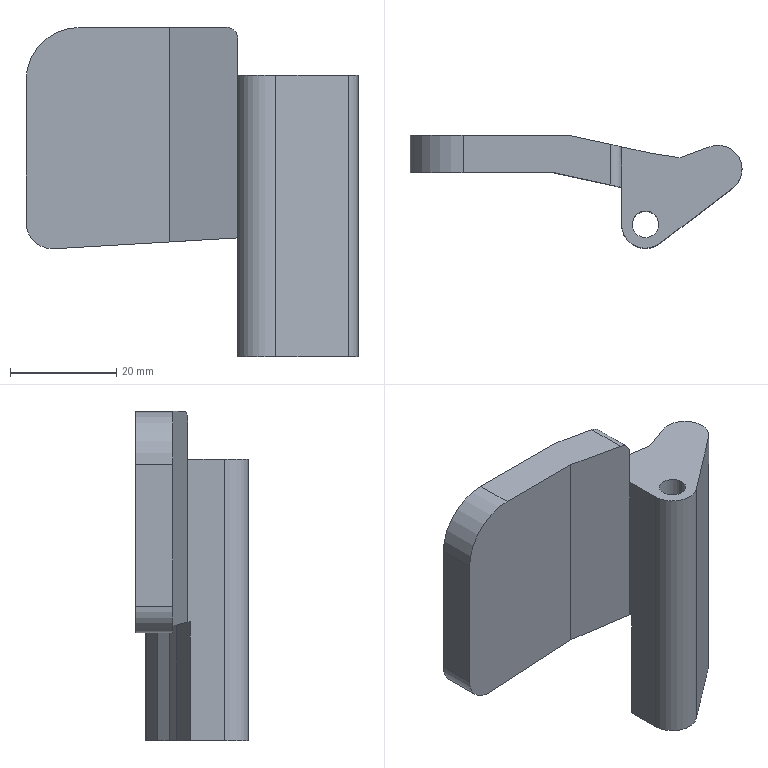Part | SolidWorks | features BaseBody 1 | 1 solid | 24 faces | box 62.54 x 21.236 x 62 mm | volume 25261 mm3 | plane 17 | cylinder 7 | commonest cylinder face diameters 5 x2 9 x2 4 x1 10 x1 20 x1
STEP:
#1=CARTESIAN_POINT('',(-2.5,0.,-26.5));
#2=VERTEX_POINT('',#1);
#3=CARTESIAN_POINT('',(2.5,0.,-26.5));
#4=VERTEX_POINT('',#3);
#5=CARTESIAN_POINT('',(0.,0.,-26.5));
#6=DIRECTION('',(0.,0.,1.));
#7=DIRECTION('',(1.,0.,0.));
#8=AXIS2_PLACEMENT_3D('',#5,#6,#7);
#9=CIRCLE('',#8,2.5);
#10=EDGE_CURVE('',#2,#4,#9,.T.);
#11=ORIENTED_EDGE('',*,*,#10,.F.);
#12=CARTESIAN_POINT('',(-2.5,0.,26.5));
#13=VERTEX_POINT('',#12);
#14=CARTESIAN_POINT('',(-2.5,0.,-26.5));
#15=DIRECTION('',(0.,0.,1.));
#16=VECTOR('',#15,1000.);
#17=LINE('',#14,#16);
#18=EDGE_CURVE('',#2,#13,#17,.T.);
#19=ORIENTED_EDGE('',*,*,#18,.T.);
#20=CARTESIAN_POINT('',(2.5,0.,26.5));
#21=VERTEX_POINT('',#20);
#22=CARTESIAN_POINT('',(0.,0.,26.5));
#23=DIRECTION('',(0.,0.,-1.));
#24=DIRECTION('',(1.,0.,0.));
#25=AXIS2_PLACEMENT_3D('',#22,#23,#24);
#26=CIRCLE('',#25,2.5);
#27=EDGE_CURVE('',#21,#13,#26,.T.);
#28=ORIENTED_EDGE('',*,*,#27,.F.);
#29=CARTESIAN_POINT('',(2.5,0.,-26.5));
#30=DIRECTION('',(0.,0.,1.));
#31=VECTOR('',#30,1000.);
#32=LINE('',#29,#31);
#33=EDGE_CURVE('',#4,#21,#32,.T.);
#34=ORIENTED_EDGE('',*,*,#33,.F.);
#35=EDGE_LOOP('',(#11,#19,#28,#34));
#36=FACE_OUTER_BOUND('',#35,.T.);
#37=CARTESIAN_POINT('',(0.,0.,-26.5));
#38=DIRECTION('',(0.,0.,1.));
#39=DIRECTION('',(1.,0.,0.));
#40=AXIS2_PLACEMENT_3D('',#37,#38,#39);
#41=CYLINDRICAL_SURFACE('',#40,2.5);
#42=ADVANCED_FACE('',(#36),#41,.F.);
#43=CARTESIAN_POINT('',(-14.348,16.736,35.5));
#44=VERTEX_POINT('',#43);
#45=CARTESIAN_POINT('',(-34.348,16.736,35.5));
#46=VERTEX_POINT('',#45);
#47=CARTESIAN_POINT('',(-14.348,16.736,35.5));
#48=DIRECTION('',(-1.,0.,0.));
#49=VECTOR('',#48,1000.);
#50=LINE('',#47,#49);
#51=EDGE_CURVE('',#44,#46,#50,.T.);
#52=ORIENTED_EDGE('',*,*,#51,.F.);
#53=CARTESIAN_POINT('',(-14.348,16.736,-4.731));
#54=VERTEX_POINT('',#53);
#55=CARTESIAN_POINT('',(-14.348,16.736,26.5));
#56=DIRECTION('',(0.,0.,1.));
#57=VECTOR('',#56,1000.);
#58=LINE('',#55,#57);
#59=EDGE_CURVE('',#54,#44,#58,.T.);
#60=ORIENTED_EDGE('',*,*,#59,.F.);
#61=CARTESIAN_POINT('',(-39.054,16.736,-6.188));
#62=VERTEX_POINT('',#61);
#63=CARTESIAN_POINT('',(-39.054,16.736,-6.188));
#64=DIRECTION('',(0.9983,0.,0.05888));
#65=VECTOR('',#64,1000.);
#66=LINE('',#63,#65);
#67=EDGE_CURVE('',#62,#54,#66,.T.);
#68=ORIENTED_EDGE('',*,*,#67,.F.);
#69=CARTESIAN_POINT('',(-44.348,16.736,-1.196));
#70=VERTEX_POINT('',#69);
#71=CARTESIAN_POINT('',(-39.348,16.736,-1.196));
#72=DIRECTION('',(0.,-1.,0.));
#73=DIRECTION('',(0.,0.,1.));
#74=AXIS2_PLACEMENT_3D('',#71,#72,#73);
#75=CIRCLE('',#74,5.);
#76=EDGE_CURVE('',#70,#62,#75,.T.);
#77=ORIENTED_EDGE('',*,*,#76,.F.);
#78=CARTESIAN_POINT('',(-44.348,16.736,25.5));
#79=VERTEX_POINT('',#78);
#80=CARTESIAN_POINT('',(-44.348,16.736,26.5));
#81=DIRECTION('',(0.,0.,-1.));
#82=VECTOR('',#81,1000.);
#83=LINE('',#80,#82);
#84=EDGE_CURVE('',#79,#70,#83,.T.);
#85=ORIENTED_EDGE('',*,*,#84,.F.);
#86=CARTESIAN_POINT('',(-34.348,16.736,25.5));
#87=DIRECTION('',(0.,-1.,0.));
#88=DIRECTION('',(0.,0.,1.));
#89=AXIS2_PLACEMENT_3D('',#86,#87,#88);
#90=CIRCLE('',#89,10.);
#91=EDGE_CURVE('',#46,#79,#90,.T.);
#92=ORIENTED_EDGE('',*,*,#91,.F.);
#93=EDGE_LOOP('',(#52,#60,#68,#77,#85,#92));
#94=FACE_OUTER_BOUND('',#93,.T.);
#95=CARTESIAN_POINT('',(-14.348,16.736,26.5));
#96=DIRECTION('',(0.,-1.,0.));
#97=DIRECTION('',(1.,0.,0.));
#98=AXIS2_PLACEMENT_3D('',#95,#96,#97);
#99=PLANE('',#98);
#100=ADVANCED_FACE('',(#94),#99,.F.);
#101=ORIENTED_EDGE('',*,*,#91,.T.);
#102=CARTESIAN_POINT('',(-44.348,9.736,25.5));
#103=VERTEX_POINT('',#102);
#104=CARTESIAN_POINT('',(-44.348,0.,25.5));
#105=DIRECTION('',(0.,-1.,0.));
#106=VECTOR('',#105,1000.);
#107=LINE('',#104,#106);
#108=EDGE_CURVE('',#79,#103,#107,.T.);
#109=ORIENTED_EDGE('',*,*,#108,.T.);
#110=CARTESIAN_POINT('',(-34.348,9.736,35.5));
#111=VERTEX_POINT('',#110);
#112=CARTESIAN_POINT('',(-34.348,9.736,25.5));
#113=DIRECTION('',(0.,1.,0.));
#114=DIRECTION('',(0.,0.,1.));
#115=AXIS2_PLACEMENT_3D('',#112,#113,#114);
#116=CIRCLE('',#115,10.);
#117=EDGE_CURVE('',#103,#111,#116,.T.);
#118=ORIENTED_EDGE('',*,*,#117,.T.);
#119=CARTESIAN_POINT('',(-34.348,0.,35.5));
#120=DIRECTION('',(0.,1.,0.));
#121=VECTOR('',#120,1000.);
#122=LINE('',#119,#121);
#123=EDGE_CURVE('',#111,#46,#122,.T.);
#124=ORIENTED_EDGE('',*,*,#123,.T.);
#125=EDGE_LOOP('',(#101,#109,#118,#124));
#126=FACE_OUTER_BOUND('',#125,.T.);
#127=CARTESIAN_POINT('',(-34.348,0.,25.5));
#128=DIRECTION('',(0.,1.,0.));
#129=DIRECTION('',(0.,0.,1.));
#130=AXIS2_PLACEMENT_3D('',#127,#128,#129);
#131=CYLINDRICAL_SURFACE('',#130,10.);
#132=ADVANCED_FACE('',(#126),#131,.T.);
#133=CARTESIAN_POINT('',(-6.5,15.04,35.5));
#134=VERTEX_POINT('',#133);
#135=CARTESIAN_POINT('',(-6.5,15.04,35.5));
#136=DIRECTION('',(-0.9774,0.2113,0.));
#137=VECTOR('',#136,1000.);
#138=LINE('',#135,#137);
#139=EDGE_CURVE('',#134,#44,#138,.T.);
#140=ORIENTED_EDGE('',*,*,#139,.T.);
#141=ORIENTED_EDGE('',*,*,#51,.T.);
#142=ORIENTED_EDGE('',*,*,#123,.F.);
#143=CARTESIAN_POINT('',(-17.348,9.736,35.5));
#144=VERTEX_POINT('',#143);
#145=CARTESIAN_POINT('',(0.,9.736,35.5));
#146=DIRECTION('',(1.,0.,0.));
#147=VECTOR('',#146,1000.);
#148=LINE('',#145,#147);
#149=EDGE_CURVE('',#111,#144,#148,.T.);
#150=ORIENTED_EDGE('',*,*,#149,.T.);
#151=CARTESIAN_POINT('',(-6.5,7.391,35.5));
#152=VERTEX_POINT('',#151);
#153=CARTESIAN_POINT('',(-17.348,9.736,35.5));
#154=DIRECTION('',(0.9774,-0.2113,0.));
#155=VECTOR('',#154,1000.);
#156=LINE('',#153,#155);
#157=EDGE_CURVE('',#144,#152,#156,.T.);
#158=ORIENTED_EDGE('',*,*,#157,.T.);
#159=CARTESIAN_POINT('',(-6.5,0.,35.5));
#160=DIRECTION('',(0.,1.,0.));
#161=VECTOR('',#160,1000.);
#162=LINE('',#159,#161);
#163=EDGE_CURVE('',#152,#134,#162,.T.);
#164=ORIENTED_EDGE('',*,*,#163,.T.);
#165=EDGE_LOOP('',(#140,#141,#142,#150,#158,#164));
#166=FACE_OUTER_BOUND('',#165,.T.);
#167=CARTESIAN_POINT('',(0.,0.,35.5));
#168=DIRECTION('',(0.,0.,1.));
#169=DIRECTION('',(1.,0.,0.));
#170=AXIS2_PLACEMENT_3D('',#167,#168,#169);
#171=PLANE('',#170);
#172=ADVANCED_FACE('',(#166),#171,.T.);
#173=CARTESIAN_POINT('',(-4.5,14.608,26.5));
#174=VERTEX_POINT('',#173);
#175=CARTESIAN_POINT('',(-4.5,14.608,33.5));
#176=VERTEX_POINT('',#175);
#177=CARTESIAN_POINT('',(-4.5,14.608,26.5));
#178=DIRECTION('',(0.,0.,1.));
#179=VECTOR('',#178,1000.);
#180=LINE('',#177,#179);
#181=EDGE_CURVE('',#174,#176,#180,.T.);
#182=ORIENTED_EDGE('',*,*,#181,.F.);
#183=CARTESIAN_POINT('',(1.316,13.35,26.5));
#184=VERTEX_POINT('',#183);
#185=CARTESIAN_POINT('',(1.316,13.35,26.5));
#186=DIRECTION('',(-0.9774,0.2113,0.));
#187=VECTOR('',#186,1000.);
#188=LINE('',#185,#187);
#189=EDGE_CURVE('',#184,#174,#188,.T.);
#190=ORIENTED_EDGE('',*,*,#189,.F.);
#191=CARTESIAN_POINT('',(1.316,13.35,-3.807));
#192=VERTEX_POINT('',#191);
#193=CARTESIAN_POINT('',(1.316,13.35,26.5));
#194=DIRECTION('',(0.,0.,1.));
#195=VECTOR('',#194,1000.);
#196=LINE('',#193,#195);
#197=EDGE_CURVE('',#192,#184,#196,.T.);
#198=ORIENTED_EDGE('',*,*,#197,.F.);
#199=CARTESIAN_POINT('',(-14.348,16.736,-4.731));
#200=DIRECTION('',(0.9758,-0.2109,0.05755));
#201=VECTOR('',#200,1000.);
#202=LINE('',#199,#201);
#203=EDGE_CURVE('',#54,#192,#202,.T.);
#204=ORIENTED_EDGE('',*,*,#203,.F.);
#205=ORIENTED_EDGE('',*,*,#59,.T.);
#206=ORIENTED_EDGE('',*,*,#139,.F.);
#207=CARTESIAN_POINT('',(-4.5,14.608,33.5));
#208=CARTESIAN_POINT('',(-4.5,14.608,34.672));
#209=CARTESIAN_POINT('',(-5.328,14.787,35.5));
#210=CARTESIAN_POINT('',(-6.5,15.04,35.5));
#211=(BOUNDED_CURVE()B_SPLINE_CURVE(3,(#207,#208,#209,#210),.UNSPECIFIED.,.F.,.T.)B_SPLINE_CURVE_WITH_KNOTS((4,4),(0.,1.571),.UNSPECIFIED.)CURVE()GEOMETRIC_REPRESENTATION_ITEM()RATIONAL_B_SPLINE_CURVE((1.,0.8047,0.8047,1.))REPRESENTATION_ITEM(''));
#212=EDGE_CURVE('',#176,#134,#211,.T.);
#213=ORIENTED_EDGE('',*,*,#212,.F.);
#214=EDGE_LOOP('',(#182,#190,#198,#204,#205,#206,#213));
#215=FACE_OUTER_BOUND('',#214,.T.);
#216=CARTESIAN_POINT('',(1.316,13.35,26.5));
#217=DIRECTION('',(-0.2113,-0.9774,0.));
#218=DIRECTION('',(0.9774,-0.2113,0.));
#219=AXIS2_PLACEMENT_3D('',#216,#217,#218);
#220=PLANE('',#219);
#221=ADVANCED_FACE('',(#215),#220,.F.);
#222=ORIENTED_EDGE('',*,*,#67,.T.);
#223=ORIENTED_EDGE('',*,*,#203,.T.);
#224=CARTESIAN_POINT('',(6.515,12.564,-3.5));
#225=VERTEX_POINT('',#224);
#226=CARTESIAN_POINT('',(6.515,12.564,-3.5));
#227=DIRECTION('',(-0.9871,0.1492,-0.05822));
#228=VECTOR('',#227,1000.);
#229=LINE('',#226,#228);
#230=EDGE_CURVE('',#225,#192,#229,.T.);
#231=ORIENTED_EDGE('',*,*,#230,.F.);
#232=CARTESIAN_POINT('',(4.675,10.439,-3.609));
#233=VERTEX_POINT('',#232);
#234=CARTESIAN_POINT('',(4.675,10.439,-3.609));
#235=DIRECTION('',(0.654,0.7555,0.03858));
#236=VECTOR('',#235,1000.);
#237=LINE('',#234,#236);
#238=EDGE_CURVE('',#233,#225,#237,.T.);
#239=ORIENTED_EDGE('',*,*,#238,.F.);
#240=CARTESIAN_POINT('',(2.605,9.013,-3.731));
#241=VERTEX_POINT('',#240);
#242=CARTESIAN_POINT('',(2.605,9.013,-3.731));
#243=DIRECTION('',(0.8226,0.5666,0.04852));
#244=VECTOR('',#243,1000.);
#245=LINE('',#242,#244);
#246=EDGE_CURVE('',#241,#233,#245,.T.);
#247=ORIENTED_EDGE('',*,*,#246,.F.);
#248=CARTESIAN_POINT('',(-4.5,6.427,-4.15));
#249=VERTEX_POINT('',#248);
#250=CARTESIAN_POINT('',(-4.5,6.427,-4.15));
#251=DIRECTION('',(0.9383,0.3415,0.05534));
#252=VECTOR('',#251,1000.);
#253=LINE('',#250,#252);
#254=EDGE_CURVE('',#249,#241,#253,.T.);
#255=ORIENTED_EDGE('',*,*,#254,.F.);
#256=CARTESIAN_POINT('',(-4.5,6.959,-4.15));
#257=VERTEX_POINT('',#256);
#258=CARTESIAN_POINT('',(-4.5,0.,-4.15));
#259=DIRECTION('',(0.,1.,0.));
#260=VECTOR('',#259,1000.);
#261=LINE('',#258,#260);
#262=EDGE_CURVE('',#249,#257,#261,.T.);
#263=ORIENTED_EDGE('',*,*,#262,.T.);
#264=CARTESIAN_POINT('',(-17.348,9.736,-4.907));
#265=VERTEX_POINT('',#264);
#266=CARTESIAN_POINT('',(-17.348,9.736,-4.907));
#267=DIRECTION('',(0.9758,-0.2109,0.05755));
#268=VECTOR('',#267,1000.);
#269=LINE('',#266,#268);
#270=EDGE_CURVE('',#265,#257,#269,.T.);
#271=ORIENTED_EDGE('',*,*,#270,.F.);
#272=CARTESIAN_POINT('',(-39.054,9.736,-6.188));
#273=VERTEX_POINT('',#272);
#274=CARTESIAN_POINT('',(-44.348,9.736,-6.5));
#275=DIRECTION('',(0.9983,0.,0.05888));
#276=VECTOR('',#275,1000.);
#277=LINE('',#274,#276);
#278=EDGE_CURVE('',#273,#265,#277,.T.);
#279=ORIENTED_EDGE('',*,*,#278,.F.);
#280=CARTESIAN_POINT('',(-39.054,-51.743,-6.188));
#281=DIRECTION('',(0.,-1.,0.));
#282=VECTOR('',#281,1000.);
#283=LINE('',#280,#282);
#284=EDGE_CURVE('',#62,#273,#283,.T.);
#285=ORIENTED_EDGE('',*,*,#284,.F.);
#286=EDGE_LOOP('',(#222,#223,#231,#239,#247,#255,#263,#271,#279,#285));
#287=FACE_OUTER_BOUND('',#286,.T.);
#288=CARTESIAN_POINT('',(-44.348,-51.743,-6.5));
#289=DIRECTION('',(-0.05888,0.,0.9983));
#290=DIRECTION('',(0.9983,0.,0.05888));
#291=AXIS2_PLACEMENT_3D('',#288,#289,#290);
#292=PLANE('',#291);
#293=ADVANCED_FACE('',(#287),#292,.F.);
#294=CARTESIAN_POINT('',(-44.348,9.736,-1.196));
#295=VERTEX_POINT('',#294);
#296=CARTESIAN_POINT('',(-39.348,9.736,-1.196));
#297=DIRECTION('',(0.,1.,0.));
#298=DIRECTION('',(0.,0.,1.));
#299=AXIS2_PLACEMENT_3D('',#296,#297,#298);
#300=CIRCLE('',#299,5.);
#301=EDGE_CURVE('',#273,#295,#300,.T.);
#302=ORIENTED_EDGE('',*,*,#301,.T.);
#303=CARTESIAN_POINT('',(-44.348,-51.743,-1.196));
#304=DIRECTION('',(0.,1.,0.));
#305=VECTOR('',#304,1000.);
#306=LINE('',#303,#305);
#307=EDGE_CURVE('',#295,#70,#306,.T.);
#308=ORIENTED_EDGE('',*,*,#307,.T.);
#309=ORIENTED_EDGE('',*,*,#76,.T.);
#310=ORIENTED_EDGE('',*,*,#284,.T.);
#311=EDGE_LOOP('',(#302,#308,#309,#310));
#312=FACE_OUTER_BOUND('',#311,.T.);
#313=CARTESIAN_POINT('',(-39.348,-51.743,-1.196));
#314=DIRECTION('',(0.,1.,0.));
#315=DIRECTION('',(0.,0.,1.));
#316=AXIS2_PLACEMENT_3D('',#313,#314,#315);
#317=CYLINDRICAL_SURFACE('',#316,5.);
#318=ADVANCED_FACE('',(#312),#317,.T.);
#319=ORIENTED_EDGE('',*,*,#84,.T.);
#320=ORIENTED_EDGE('',*,*,#307,.F.);
#321=CARTESIAN_POINT('',(-44.348,9.736,26.5));
#322=DIRECTION('',(0.,0.,-1.));
#323=VECTOR('',#322,1000.);
#324=LINE('',#321,#323);
#325=EDGE_CURVE('',#103,#295,#324,.T.);
#326=ORIENTED_EDGE('',*,*,#325,.F.);
#327=ORIENTED_EDGE('',*,*,#108,.F.);
#328=EDGE_LOOP('',(#319,#320,#326,#327));
#329=FACE_OUTER_BOUND('',#328,.T.);
#330=CARTESIAN_POINT('',(-44.348,16.736,26.5));
#331=DIRECTION('',(1.,0.,0.));
#332=DIRECTION('',(0.,0.,-1.));
#333=AXIS2_PLACEMENT_3D('',#330,#331,#332);
#334=PLANE('',#333);
#335=ADVANCED_FACE('',(#329),#334,.F.);
#336=ORIENTED_EDGE('',*,*,#325,.T.);
#337=ORIENTED_EDGE('',*,*,#301,.F.);
#338=ORIENTED_EDGE('',*,*,#278,.T.);
#339=CARTESIAN_POINT('',(-17.348,9.736,26.5));
#340=DIRECTION('',(0.,0.,-1.));
#341=VECTOR('',#340,1000.);
#342=LINE('',#339,#341);
#343=EDGE_CURVE('',#144,#265,#342,.T.);
#344=ORIENTED_EDGE('',*,*,#343,.F.);
#345=ORIENTED_EDGE('',*,*,#149,.F.);
#346=ORIENTED_EDGE('',*,*,#117,.F.);
#347=EDGE_LOOP('',(#336,#337,#338,#344,#345,#346));
#348=FACE_OUTER_BOUND('',#347,.T.);
#349=CARTESIAN_POINT('',(-44.348,9.736,26.5));
#350=DIRECTION('',(0.,1.,0.));
#351=DIRECTION('',(-1.,0.,0.));
#352=AXIS2_PLACEMENT_3D('',#349,#350,#351);
#353=PLANE('',#352);
#354=ADVANCED_FACE('',(#348),#353,.F.);
#355=CARTESIAN_POINT('',(-4.5,6.959,33.5));
#356=VERTEX_POINT('',#355);
#357=CARTESIAN_POINT('',(-6.5,7.391,35.5));
#358=CARTESIAN_POINT('',(-5.328,7.138,35.5));
#359=CARTESIAN_POINT('',(-4.5,6.959,34.672));
#360=CARTESIAN_POINT('',(-4.5,6.959,33.5));
#361=(BOUNDED_CURVE()B_SPLINE_CURVE(3,(#357,#358,#359,#360),.UNSPECIFIED.,.F.,.F.)B_SPLINE_CURVE_WITH_KNOTS((4,4),(4.712,6.283),.UNSPECIFIED.)CURVE()GEOMETRIC_REPRESENTATION_ITEM()RATIONAL_B_SPLINE_CURVE((1.,0.8047,0.8047,1.))REPRESENTATION_ITEM(''));
#362=EDGE_CURVE('',#152,#356,#361,.T.);
#363=ORIENTED_EDGE('',*,*,#362,.T.);
#364=CARTESIAN_POINT('',(-4.5,0.,33.5));
#365=DIRECTION('',(0.,1.,0.));
#366=VECTOR('',#365,1000.);
#367=LINE('',#364,#366);
#368=EDGE_CURVE('',#356,#176,#367,.T.);
#369=ORIENTED_EDGE('',*,*,#368,.T.);
#370=ORIENTED_EDGE('',*,*,#212,.T.);
#371=ORIENTED_EDGE('',*,*,#163,.F.);
#372=EDGE_LOOP('',(#363,#369,#370,#371));
#373=FACE_OUTER_BOUND('',#372,.T.);
#374=CARTESIAN_POINT('',(-6.5,0.,33.5));
#375=DIRECTION('',(0.,-1.,0.));
#376=DIRECTION('',(0.,0.,-1.));
#377=AXIS2_PLACEMENT_3D('',#374,#375,#376);
#378=CYLINDRICAL_SURFACE('',#377,2.);
#379=ADVANCED_FACE('',(#373),#378,.T.);
#380=ORIENTED_EDGE('',*,*,#157,.F.);
#381=ORIENTED_EDGE('',*,*,#343,.T.);
#382=ORIENTED_EDGE('',*,*,#270,.T.);
#383=CARTESIAN_POINT('',(-4.5,6.959,26.5));
#384=VERTEX_POINT('',#383);
#385=CARTESIAN_POINT('',(-4.5,6.959,26.5));
#386=DIRECTION('',(0.,0.,-1.));
#387=VECTOR('',#386,1000.);
#388=LINE('',#385,#387);
#389=EDGE_CURVE('',#384,#257,#388,.T.);
#390=ORIENTED_EDGE('',*,*,#389,.F.);
#391=CARTESIAN_POINT('',(-4.5,6.959,26.5));
#392=DIRECTION('',(0.,0.,-1.));
#393=VECTOR('',#392,1000.);
#394=LINE('',#391,#393);
#395=EDGE_CURVE('',#356,#384,#394,.T.);
#396=ORIENTED_EDGE('',*,*,#395,.F.);
#397=ORIENTED_EDGE('',*,*,#362,.F.);
#398=EDGE_LOOP('',(#380,#381,#382,#390,#396,#397));
#399=FACE_OUTER_BOUND('',#398,.T.);
#400=CARTESIAN_POINT('',(-17.348,9.736,26.5));
#401=DIRECTION('',(0.2113,0.9774,0.));
#402=DIRECTION('',(-0.9774,0.2113,0.));
#403=AXIS2_PLACEMENT_3D('',#400,#401,#402);
#404=PLANE('',#403);
#405=ADVANCED_FACE('',(#399),#404,.F.);
#406=ORIENTED_EDGE('',*,*,#395,.T.);
#407=CARTESIAN_POINT('',(-4.5,6.959,26.5));
#408=DIRECTION('',(0.,-1.,0.));
#409=VECTOR('',#408,1000.);
#410=LINE('',#407,#409);
#411=EDGE_CURVE('',#174,#384,#410,.T.);
#412=ORIENTED_EDGE('',*,*,#411,.F.);
#413=ORIENTED_EDGE('',*,*,#181,.T.);
#414=ORIENTED_EDGE('',*,*,#368,.F.);
#415=EDGE_LOOP('',(#406,#412,#413,#414));
#416=FACE_OUTER_BOUND('',#415,.T.);
#417=CARTESIAN_POINT('',(-4.5,6.959,35.5));
#418=DIRECTION('',(-1.,0.,0.));
#419=DIRECTION('',(0.,0.,1.));
#420=AXIS2_PLACEMENT_3D('',#417,#418,#419);
#421=PLANE('',#420);
#422=ADVANCED_FACE('',(#416),#421,.F.);
#423=ORIENTED_EDGE('',*,*,#27,.T.);
#424=CARTESIAN_POINT('',(0.,0.,26.5));
#425=DIRECTION('',(0.,0.,-1.));
#426=DIRECTION('',(1.,0.,0.));
#427=AXIS2_PLACEMENT_3D('',#424,#425,#426);
#428=CIRCLE('',#427,2.5);
#429=EDGE_CURVE('',#13,#21,#428,.T.);
#430=ORIENTED_EDGE('',*,*,#429,.T.);
#431=EDGE_LOOP('',(#423,#430));
#432=FACE_BOUND('',#431,.T.);
#433=CARTESIAN_POINT('',(16.412,6.803,26.5));
#434=VERTEX_POINT('',#433);
#435=CARTESIAN_POINT('',(12.153,14.617,26.5));
#436=VERTEX_POINT('',#435);
#437=CARTESIAN_POINT('',(13.692,10.388,26.5));
#438=DIRECTION('',(0.,0.,1.));
#439=DIRECTION('',(-1.,0.,0.));
#440=AXIS2_PLACEMENT_3D('',#437,#438,#439);
#441=CIRCLE('',#440,4.5);
#442=EDGE_CURVE('',#434,#436,#441,.T.);
#443=ORIENTED_EDGE('',*,*,#442,.T.);
#444=CARTESIAN_POINT('',(6.515,12.564,26.5));
#445=VERTEX_POINT('',#444);
#446=CARTESIAN_POINT('',(12.153,14.617,26.5));
#447=DIRECTION('',(-0.9397,-0.342,0.));
#448=VECTOR('',#447,1000.);
#449=LINE('',#446,#448);
#450=EDGE_CURVE('',#436,#445,#449,.T.);
#451=ORIENTED_EDGE('',*,*,#450,.T.);
#452=CARTESIAN_POINT('',(6.515,12.564,26.5));
#453=DIRECTION('',(-0.9888,0.1495,0.));
#454=VECTOR('',#453,1000.);
#455=LINE('',#452,#454);
#456=EDGE_CURVE('',#445,#184,#455,.T.);
#457=ORIENTED_EDGE('',*,*,#456,.T.);
#458=ORIENTED_EDGE('',*,*,#189,.T.);
#459=ORIENTED_EDGE('',*,*,#411,.T.);
#460=CARTESIAN_POINT('',(-4.5,0.,26.5));
#461=VERTEX_POINT('',#460);
#462=CARTESIAN_POINT('',(-4.5,0.,26.5));
#463=DIRECTION('',(0.,-1.,0.));
#464=VECTOR('',#463,1000.);
#465=LINE('',#462,#464);
#466=EDGE_CURVE('',#384,#461,#465,.T.);
#467=ORIENTED_EDGE('',*,*,#466,.T.);
#468=CARTESIAN_POINT('',(2.7,-3.6,26.5));
#469=VERTEX_POINT('',#468);
#470=CARTESIAN_POINT('',(0.,0.,26.5));
#471=DIRECTION('',(0.,0.,1.));
#472=DIRECTION('',(-1.,0.,0.));
#473=AXIS2_PLACEMENT_3D('',#470,#471,#472);
#474=CIRCLE('',#473,4.5);
#475=EDGE_CURVE('',#461,#469,#474,.T.);
#476=ORIENTED_EDGE('',*,*,#475,.T.);
#477=CARTESIAN_POINT('',(2.7,-3.6,26.5));
#478=DIRECTION('',(0.7967,0.6044,0.));
#479=VECTOR('',#478,1000.);
#480=LINE('',#477,#479);
#481=EDGE_CURVE('',#469,#434,#480,.T.);
#482=ORIENTED_EDGE('',*,*,#481,.T.);
#483=EDGE_LOOP('',(#443,#451,#457,#458,#459,#467,#476,#482));
#484=FACE_OUTER_BOUND('',#483,.T.);
#485=CARTESIAN_POINT('',(0.,0.,26.5));
#486=DIRECTION('',(0.,0.,1.));
#487=DIRECTION('',(1.,0.,0.));
#488=AXIS2_PLACEMENT_3D('',#485,#486,#487);
#489=PLANE('',#488);
#490=ADVANCED_FACE('',(#432,#484),#489,.T.);
#491=ORIENTED_EDGE('',*,*,#197,.T.);
#492=ORIENTED_EDGE('',*,*,#456,.F.);
#493=CARTESIAN_POINT('',(6.515,12.564,26.5));
#494=DIRECTION('',(0.,0.,1.));
#495=VECTOR('',#494,1000.);
#496=LINE('',#493,#495);
#497=EDGE_CURVE('',#225,#445,#496,.T.);
#498=ORIENTED_EDGE('',*,*,#497,.F.);
#499=ORIENTED_EDGE('',*,*,#230,.T.);
#500=EDGE_LOOP('',(#491,#492,#498,#499));
#501=FACE_OUTER_BOUND('',#500,.T.);
#502=CARTESIAN_POINT('',(1.316,13.35,26.5));
#503=DIRECTION('',(-0.1495,-0.9888,0.));
#504=DIRECTION('',(0.9888,-0.1495,0.));
#505=AXIS2_PLACEMENT_3D('',#502,#503,#504);
#506=PLANE('',#505);
#507=ADVANCED_FACE('',(#501),#506,.F.);
#508=CARTESIAN_POINT('',(6.515,12.564,-26.5));
#509=VERTEX_POINT('',#508);
#510=CARTESIAN_POINT('',(6.515,12.564,-6.5));
#511=DIRECTION('',(0.,0.,1.));
#512=VECTOR('',#511,1000.);
#513=LINE('',#510,#512);
#514=EDGE_CURVE('',#509,#225,#513,.T.);
#515=ORIENTED_EDGE('',*,*,#514,.F.);
#516=CARTESIAN_POINT('',(4.675,10.439,-26.5));
#517=VERTEX_POINT('',#516);
#518=CARTESIAN_POINT('',(6.515,12.564,-26.5));
#519=DIRECTION('',(0.6545,0.7561,0.));
#520=VECTOR('',#519,1000.);
#521=LINE('',#518,#520);
#522=EDGE_CURVE('',#517,#509,#521,.T.);
#523=ORIENTED_EDGE('',*,*,#522,.F.);
#524=CARTESIAN_POINT('',(4.675,10.439,-6.5));
#525=DIRECTION('',(0.,0.,-1.));
#526=VECTOR('',#525,1000.);
#527=LINE('',#524,#526);
#528=EDGE_CURVE('',#233,#517,#527,.T.);
#529=ORIENTED_EDGE('',*,*,#528,.F.);
#530=ORIENTED_EDGE('',*,*,#238,.T.);
#531=EDGE_LOOP('',(#515,#523,#529,#530));
#532=FACE_OUTER_BOUND('',#531,.T.);
#533=CARTESIAN_POINT('',(6.515,12.564,-6.5));
#534=DIRECTION('',(0.7561,-0.6545,0.));
#535=DIRECTION('',(0.6545,0.7561,0.));
#536=AXIS2_PLACEMENT_3D('',#533,#534,#535);
#537=PLANE('',#536);
#538=ADVANCED_FACE('',(#532),#537,.F.);
#539=ORIENTED_EDGE('',*,*,#528,.T.);
#540=CARTESIAN_POINT('',(2.605,9.013,-26.5));
#541=VERTEX_POINT('',#540);
#542=CARTESIAN_POINT('',(4.675,10.439,-26.5));
#543=DIRECTION('',(0.8235,0.5673,0.));
#544=VECTOR('',#543,1000.);
#545=LINE('',#542,#544);
#546=EDGE_CURVE('',#541,#517,#545,.T.);
#547=ORIENTED_EDGE('',*,*,#546,.F.);
#548=CARTESIAN_POINT('',(2.605,9.013,-6.5));
#549=DIRECTION('',(0.,0.,-1.));
#550=VECTOR('',#549,1000.);
#551=LINE('',#548,#550);
#552=EDGE_CURVE('',#241,#541,#551,.T.);
#553=ORIENTED_EDGE('',*,*,#552,.F.);
#554=ORIENTED_EDGE('',*,*,#246,.T.);
#555=EDGE_LOOP('',(#539,#547,#553,#554));
#556=FACE_OUTER_BOUND('',#555,.T.);
#557=CARTESIAN_POINT('',(4.675,10.439,-6.5));
#558=DIRECTION('',(0.5673,-0.8235,0.));
#559=DIRECTION('',(0.8235,0.5673,0.));
#560=AXIS2_PLACEMENT_3D('',#557,#558,#559);
#561=PLANE('',#560);
#562=ADVANCED_FACE('',(#556),#561,.F.);
#563=CARTESIAN_POINT('',(-4.5,6.427,-26.5));
#564=VERTEX_POINT('',#563);
#565=CARTESIAN_POINT('',(2.605,9.013,-26.5));
#566=DIRECTION('',(0.9397,0.342,0.));
#567=VECTOR('',#566,1000.);
#568=LINE('',#565,#567);
#569=EDGE_CURVE('',#564,#541,#568,.T.);
#570=ORIENTED_EDGE('',*,*,#569,.F.);
#571=CARTESIAN_POINT('',(-4.5,6.427,-6.5));
#572=DIRECTION('',(0.,0.,-1.));
#573=VECTOR('',#572,1000.);
#574=LINE('',#571,#573);
#575=EDGE_CURVE('',#249,#564,#574,.T.);
#576=ORIENTED_EDGE('',*,*,#575,.F.);
#577=ORIENTED_EDGE('',*,*,#254,.T.);
#578=ORIENTED_EDGE('',*,*,#552,.T.);
#579=EDGE_LOOP('',(#570,#576,#577,#578));
#580=FACE_OUTER_BOUND('',#579,.T.);
#581=CARTESIAN_POINT('',(2.605,9.013,-6.5));
#582=DIRECTION('',(0.342,-0.9397,0.));
#583=DIRECTION('',(0.9397,0.342,0.));
#584=AXIS2_PLACEMENT_3D('',#581,#582,#583);
#585=PLANE('',#584);
#586=ADVANCED_FACE('',(#580),#585,.F.);
#587=CARTESIAN_POINT('',(-4.5,0.,-26.5));
#588=VERTEX_POINT('',#587);
#589=CARTESIAN_POINT('',(-4.5,0.,-26.5));
#590=DIRECTION('',(0.,1.,0.));
#591=VECTOR('',#590,1000.);
#592=LINE('',#589,#591);
#593=EDGE_CURVE('',#588,#564,#592,.T.);
#594=ORIENTED_EDGE('',*,*,#593,.F.);
#595=CARTESIAN_POINT('',(-4.5,0.,26.5));
#596=DIRECTION('',(0.,0.,-1.));
#597=VECTOR('',#596,1000.);
#598=LINE('',#595,#597);
#599=EDGE_CURVE('',#461,#588,#598,.T.);
#600=ORIENTED_EDGE('',*,*,#599,.F.);
#601=ORIENTED_EDGE('',*,*,#466,.F.);
#602=ORIENTED_EDGE('',*,*,#389,.T.);
#603=ORIENTED_EDGE('',*,*,#262,.F.);
#604=ORIENTED_EDGE('',*,*,#575,.T.);
#605=EDGE_LOOP('',(#594,#600,#601,#602,#603,#604));
#606=FACE_OUTER_BOUND('',#605,.T.);
#607=CARTESIAN_POINT('',(-4.5,0.,26.5));
#608=DIRECTION('',(1.,0.,0.));
#609=DIRECTION('',(0.,1.,0.));
#610=AXIS2_PLACEMENT_3D('',#607,#608,#609);
#611=PLANE('',#610);
#612=ADVANCED_FACE('',(#606),#611,.F.);
#613=ORIENTED_EDGE('',*,*,#18,.F.);
#614=CARTESIAN_POINT('',(0.,0.,-26.5));
#615=DIRECTION('',(0.,0.,1.));
#616=DIRECTION('',(1.,0.,0.));
#617=AXIS2_PLACEMENT_3D('',#614,#615,#616);
#618=CIRCLE('',#617,2.5);
#619=EDGE_CURVE('',#4,#2,#618,.T.);
#620=ORIENTED_EDGE('',*,*,#619,.F.);
#621=ORIENTED_EDGE('',*,*,#33,.T.);
#622=ORIENTED_EDGE('',*,*,#429,.F.);
#623=EDGE_LOOP('',(#613,#620,#621,#622));
#624=FACE_OUTER_BOUND('',#623,.T.);
#625=CARTESIAN_POINT('',(0.,0.,-26.5));
#626=DIRECTION('',(0.,0.,1.));
#627=DIRECTION('',(1.,0.,0.));
#628=AXIS2_PLACEMENT_3D('',#625,#626,#627);
#629=CYLINDRICAL_SURFACE('',#628,2.5);
#630=ADVANCED_FACE('',(#624),#629,.F.);
#631=ORIENTED_EDGE('',*,*,#497,.T.);
#632=ORIENTED_EDGE('',*,*,#450,.F.);
#633=CARTESIAN_POINT('',(12.153,14.617,-26.5));
#634=VERTEX_POINT('',#633);
#635=CARTESIAN_POINT('',(12.153,14.617,26.5));
#636=DIRECTION('',(0.,0.,1.));
#637=VECTOR('',#636,1000.);
#638=LINE('',#635,#637);
#639=EDGE_CURVE('',#634,#436,#638,.T.);
#640=ORIENTED_EDGE('',*,*,#639,.F.);
#641=CARTESIAN_POINT('',(6.515,12.564,-26.5));
#642=DIRECTION('',(0.9397,0.342,0.));
#643=VECTOR('',#642,1000.);
#644=LINE('',#641,#643);
#645=EDGE_CURVE('',#509,#634,#644,.T.);
#646=ORIENTED_EDGE('',*,*,#645,.F.);
#647=ORIENTED_EDGE('',*,*,#514,.T.);
#648=EDGE_LOOP('',(#631,#632,#640,#646,#647));
#649=FACE_OUTER_BOUND('',#648,.T.);
#650=CARTESIAN_POINT('',(6.515,12.564,26.5));
#651=DIRECTION('',(0.342,-0.9397,0.));
#652=DIRECTION('',(0.9397,0.342,0.));
#653=AXIS2_PLACEMENT_3D('',#650,#651,#652);
#654=PLANE('',#653);
#655=ADVANCED_FACE('',(#649),#654,.F.);
#656=CARTESIAN_POINT('',(16.412,6.803,-26.5));
#657=VERTEX_POINT('',#656);
#658=CARTESIAN_POINT('',(13.692,10.388,-26.5));
#659=DIRECTION('',(0.,0.,1.));
#660=DIRECTION('',(-1.,0.,0.));
#661=AXIS2_PLACEMENT_3D('',#658,#659,#660);
#662=CIRCLE('',#661,4.5);
#663=EDGE_CURVE('',#657,#634,#662,.T.);
#664=ORIENTED_EDGE('',*,*,#663,.T.);
#665=ORIENTED_EDGE('',*,*,#639,.T.);
#666=ORIENTED_EDGE('',*,*,#442,.F.);
#667=CARTESIAN_POINT('',(16.412,6.803,26.5));
#668=DIRECTION('',(0.,0.,-1.));
#669=VECTOR('',#668,1000.);
#670=LINE('',#667,#669);
#671=EDGE_CURVE('',#434,#657,#670,.T.);
#672=ORIENTED_EDGE('',*,*,#671,.T.);
#673=EDGE_LOOP('',(#664,#665,#666,#672));
#674=FACE_OUTER_BOUND('',#673,.T.);
#675=CARTESIAN_POINT('',(13.692,10.388,26.5));
#676=DIRECTION('',(0.,0.,-1.));
#677=DIRECTION('',(-1.,0.,0.));
#678=AXIS2_PLACEMENT_3D('',#675,#676,#677);
#679=CYLINDRICAL_SURFACE('',#678,4.5);
#680=ADVANCED_FACE('',(#674),#679,.T.);
#681=ORIENTED_EDGE('',*,*,#481,.F.);
#682=CARTESIAN_POINT('',(2.7,-3.6,-26.5));
#683=VERTEX_POINT('',#682);
#684=CARTESIAN_POINT('',(2.7,-3.6,26.5));
#685=DIRECTION('',(0.,0.,1.));
#686=VECTOR('',#685,1000.);
#687=LINE('',#684,#686);
#688=EDGE_CURVE('',#683,#469,#687,.T.);
#689=ORIENTED_EDGE('',*,*,#688,.F.);
#690=CARTESIAN_POINT('',(2.7,-3.6,-26.5));
#691=DIRECTION('',(-0.7967,-0.6044,0.));
#692=VECTOR('',#691,1000.);
#693=LINE('',#690,#692);
#694=EDGE_CURVE('',#657,#683,#693,.T.);
#695=ORIENTED_EDGE('',*,*,#694,.F.);
#696=ORIENTED_EDGE('',*,*,#671,.F.);
#697=EDGE_LOOP('',(#681,#689,#695,#696));
#698=FACE_OUTER_BOUND('',#697,.T.);
#699=CARTESIAN_POINT('',(2.7,-3.6,26.5));
#700=DIRECTION('',(-0.6044,0.7967,0.));
#701=DIRECTION('',(-0.7967,-0.6044,0.));
#702=AXIS2_PLACEMENT_3D('',#699,#700,#701);
#703=PLANE('',#702);
#704=ADVANCED_FACE('',(#698),#703,.F.);
#705=CARTESIAN_POINT('',(0.,0.,-26.5));
#706=DIRECTION('',(0.,0.,1.));
#707=DIRECTION('',(-1.,0.,0.));
#708=AXIS2_PLACEMENT_3D('',#705,#706,#707);
#709=CIRCLE('',#708,4.5);
#710=EDGE_CURVE('',#588,#683,#709,.T.);
#711=ORIENTED_EDGE('',*,*,#710,.T.);
#712=ORIENTED_EDGE('',*,*,#688,.T.);
#713=ORIENTED_EDGE('',*,*,#475,.F.);
#714=ORIENTED_EDGE('',*,*,#599,.T.);
#715=EDGE_LOOP('',(#711,#712,#713,#714));
#716=FACE_OUTER_BOUND('',#715,.T.);
#717=CARTESIAN_POINT('',(0.,0.,26.5));
#718=DIRECTION('',(0.,0.,-1.));
#719=DIRECTION('',(-1.,0.,0.));
#720=AXIS2_PLACEMENT_3D('',#717,#718,#719);
#721=CYLINDRICAL_SURFACE('',#720,4.5);
#722=ADVANCED_FACE('',(#716),#721,.T.);
#723=ORIENTED_EDGE('',*,*,#619,.T.);
#724=ORIENTED_EDGE('',*,*,#10,.T.);
#725=EDGE_LOOP('',(#723,#724));
#726=FACE_BOUND('',#725,.T.);
#727=ORIENTED_EDGE('',*,*,#546,.T.);
#728=ORIENTED_EDGE('',*,*,#522,.T.);
#729=ORIENTED_EDGE('',*,*,#645,.T.);
#730=ORIENTED_EDGE('',*,*,#663,.F.);
#731=ORIENTED_EDGE('',*,*,#694,.T.);
#732=ORIENTED_EDGE('',*,*,#710,.F.);
#733=ORIENTED_EDGE('',*,*,#593,.T.);
#734=ORIENTED_EDGE('',*,*,#569,.T.);
#735=EDGE_LOOP('',(#727,#728,#729,#730,#731,#732,#733,#734));
#736=FACE_OUTER_BOUND('',#735,.T.);
#737=CARTESIAN_POINT('',(0.,0.,-26.5));
#738=DIRECTION('',(0.,0.,1.));
#739=DIRECTION('',(1.,0.,0.));
#740=AXIS2_PLACEMENT_3D('',#737,#738,#739);
#741=PLANE('',#740);
#742=ADVANCED_FACE('',(#726,#736),#741,.F.);
#743=CLOSED_SHELL('',(#42,#100,#132,#172,#221,#293,#318,#335,#354,#379,#405,#422,#490,#507,#538,#562,#586,#612,#630,#655,#680,#704,#722,#742));
#744=MANIFOLD_SOLID_BREP('',#743);
#745=CARTESIAN_POINT('',(0.,0.,0.));
#746=DIRECTION('',(0.,0.,1.));
#747=DIRECTION('',(1.,0.,0.));
#748=AXIS2_PLACEMENT_3D('',#745,#746,#747);
#749=(LENGTH_UNIT()NAMED_UNIT(*)SI_UNIT(.MILLI.,.METRE.));
#750=UNCERTAINTY_MEASURE_WITH_UNIT(LENGTH_MEASURE(0.00001),#749,'','');
#751=(NAMED_UNIT(*)PLANE_ANGLE_UNIT()SI_UNIT($,.RADIAN.));
#752=(NAMED_UNIT(*)SI_UNIT($,.STERADIAN.)SOLID_ANGLE_UNIT());
#753=(GEOMETRIC_REPRESENTATION_CONTEXT(3)GLOBAL_UNCERTAINTY_ASSIGNED_CONTEXT((#750))GLOBAL_UNIT_ASSIGNED_CONTEXT((#749,#751,#752))REPRESENTATION_CONTEXT('',''));
#754=ADVANCED_BREP_SHAPE_REPRESENTATION('',(#744,#748),#753);